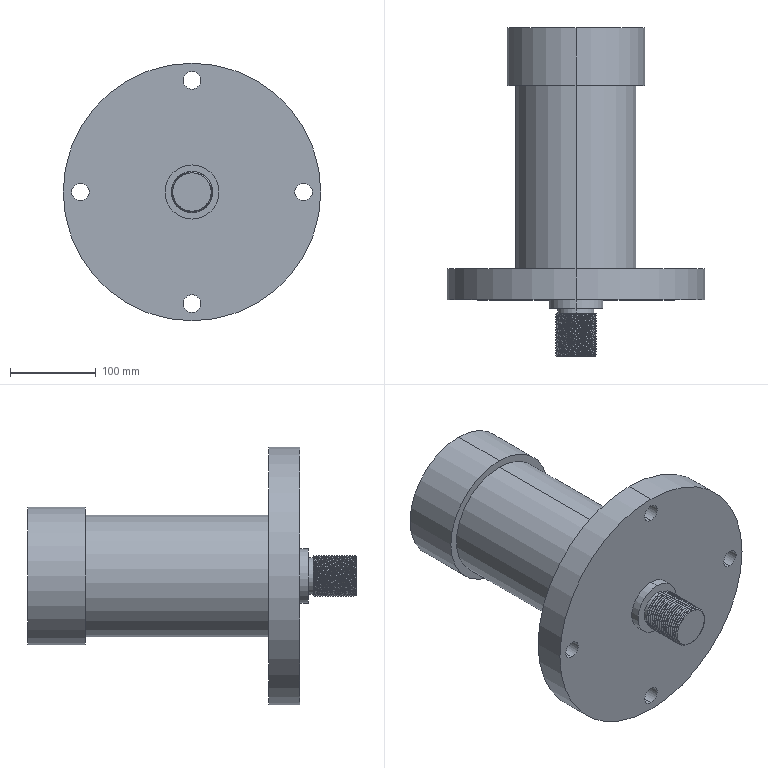Part | SolidWorks | features BaseBody 1 | 1 solid | 65 faces | box 300 x 382.79 x 300 mm | volume 7334262 mm3 | cylinder 52 | plane 7 | cone 3 | spline 3 | commonest cylinder face diameters 48 x34 20.5 x8 42.59 x2 63 x2 141.51 x2 160 x2